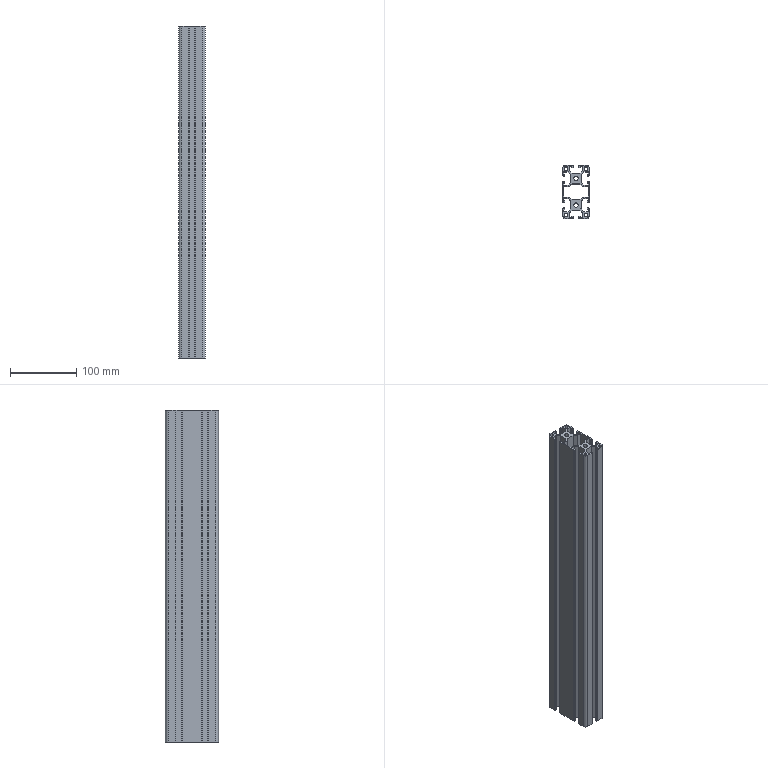Part | SolidWorks | features BaseBody 1 | 1 solid | 155 faces | box 40.002 x 80 x 500 mm | volume 492196 mm3 | plane 142 | cylinder 13 | commonest cylinder face diameters 9 x5 5 x4 6.8 x4